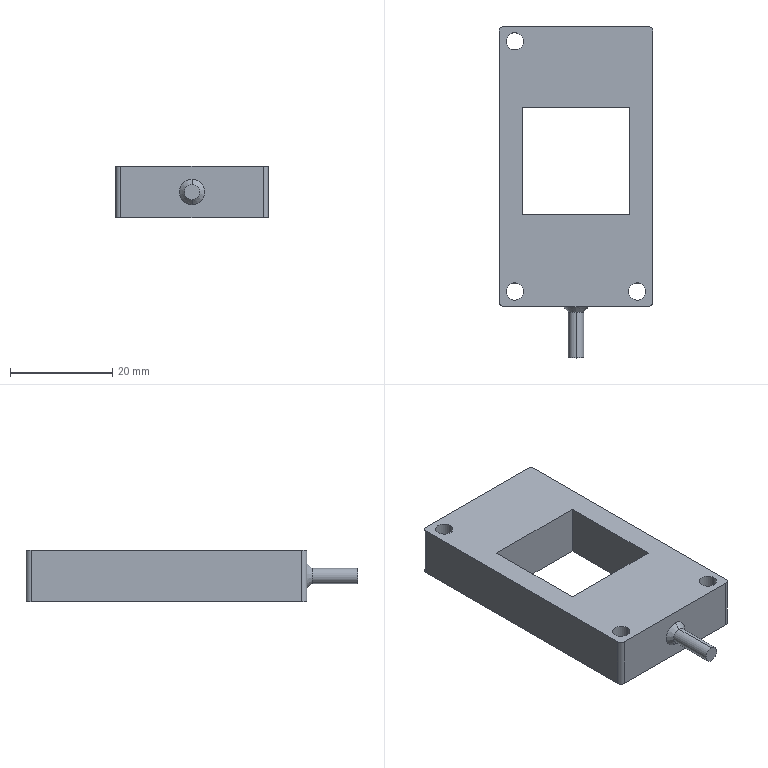Part | SolidWorks | features ICE 2, Chamfer 1, Extrusion 1, Fillet 1, HoleWzd 1 | 1 solid | 25 faces | box 30 x 65 x 10 mm | volume 11885 mm3 | cylinder 12 | plane 11 | cone 2 | commonest cylinder face diameters 3.4 x6 2 x4 3 x2
STEP:
#1=CARTESIAN_POINT('',(-13.7,24.5,-5.));
#2=VERTEX_POINT('',#1);
#3=CARTESIAN_POINT('',(-10.3,24.5,-5.));
#4=VERTEX_POINT('',#3);
#5=CARTESIAN_POINT('',(-12.,24.5,-5.));
#6=DIRECTION('',(0.,0.,1.));
#7=DIRECTION('',(1.,0.,0.));
#8=AXIS2_PLACEMENT_3D('',#5,#6,#7);
#9=CIRCLE('',#8,1.7);
#10=EDGE_CURVE('',#2,#4,#9,.T.);
#11=ORIENTED_EDGE('',*,*,#10,.F.);
#12=CARTESIAN_POINT('',(-13.7,24.5,5.));
#13=VERTEX_POINT('',#12);
#14=CARTESIAN_POINT('',(-13.7,24.5,5.));
#15=DIRECTION('',(0.,0.,1.));
#16=VECTOR('',#15,1000.);
#17=LINE('',#14,#16);
#18=EDGE_CURVE('',#2,#13,#17,.T.);
#19=ORIENTED_EDGE('',*,*,#18,.T.);
#20=CARTESIAN_POINT('',(-10.3,24.5,5.));
#21=VERTEX_POINT('',#20);
#22=CARTESIAN_POINT('',(-12.,24.5,5.));
#23=DIRECTION('',(0.,0.,1.));
#24=DIRECTION('',(1.,0.,0.));
#25=AXIS2_PLACEMENT_3D('',#22,#23,#24);
#26=CIRCLE('',#25,1.7);
#27=EDGE_CURVE('',#13,#21,#26,.T.);
#28=ORIENTED_EDGE('',*,*,#27,.T.);
#29=CARTESIAN_POINT('',(-10.3,24.5,5.));
#30=DIRECTION('',(0.,0.,1.));
#31=VECTOR('',#30,1000.);
#32=LINE('',#29,#31);
#33=EDGE_CURVE('',#4,#21,#32,.T.);
#34=ORIENTED_EDGE('',*,*,#33,.F.);
#35=EDGE_LOOP('',(#11,#19,#28,#34));
#36=FACE_OUTER_BOUND('',#35,.T.);
#37=CARTESIAN_POINT('',(-12.,24.5,5.));
#38=DIRECTION('',(0.,0.,1.));
#39=DIRECTION('',(1.,0.,0.));
#40=AXIS2_PLACEMENT_3D('',#37,#38,#39);
#41=CYLINDRICAL_SURFACE('',#40,1.7);
#42=ADVANCED_FACE('',(#36),#41,.F.);
#43=CARTESIAN_POINT('',(-13.7,-24.5,-5.));
#44=VERTEX_POINT('',#43);
#45=CARTESIAN_POINT('',(-10.3,-24.5,-5.));
#46=VERTEX_POINT('',#45);
#47=CARTESIAN_POINT('',(-12.,-24.5,-5.));
#48=DIRECTION('',(0.,0.,1.));
#49=DIRECTION('',(1.,0.,0.));
#50=AXIS2_PLACEMENT_3D('',#47,#48,#49);
#51=CIRCLE('',#50,1.7);
#52=EDGE_CURVE('',#44,#46,#51,.T.);
#53=ORIENTED_EDGE('',*,*,#52,.F.);
#54=CARTESIAN_POINT('',(-13.7,-24.5,5.));
#55=VERTEX_POINT('',#54);
#56=CARTESIAN_POINT('',(-13.7,-24.5,5.));
#57=DIRECTION('',(0.,0.,1.));
#58=VECTOR('',#57,1000.);
#59=LINE('',#56,#58);
#60=EDGE_CURVE('',#44,#55,#59,.T.);
#61=ORIENTED_EDGE('',*,*,#60,.T.);
#62=CARTESIAN_POINT('',(-10.3,-24.5,5.));
#63=VERTEX_POINT('',#62);
#64=CARTESIAN_POINT('',(-12.,-24.5,5.));
#65=DIRECTION('',(0.,0.,1.));
#66=DIRECTION('',(1.,0.,0.));
#67=AXIS2_PLACEMENT_3D('',#64,#65,#66);
#68=CIRCLE('',#67,1.7);
#69=EDGE_CURVE('',#55,#63,#68,.T.);
#70=ORIENTED_EDGE('',*,*,#69,.T.);
#71=CARTESIAN_POINT('',(-10.3,-24.5,5.));
#72=DIRECTION('',(0.,0.,1.));
#73=VECTOR('',#72,1000.);
#74=LINE('',#71,#73);
#75=EDGE_CURVE('',#46,#63,#74,.T.);
#76=ORIENTED_EDGE('',*,*,#75,.F.);
#77=EDGE_LOOP('',(#53,#61,#70,#76));
#78=FACE_OUTER_BOUND('',#77,.T.);
#79=CARTESIAN_POINT('',(-12.,-24.5,5.));
#80=DIRECTION('',(0.,0.,1.));
#81=DIRECTION('',(1.,0.,0.));
#82=AXIS2_PLACEMENT_3D('',#79,#80,#81);
#83=CYLINDRICAL_SURFACE('',#82,1.7);
#84=ADVANCED_FACE('',(#78),#83,.F.);
#85=CARTESIAN_POINT('',(10.3,-24.5,-5.));
#86=VERTEX_POINT('',#85);
#87=CARTESIAN_POINT('',(13.7,-24.5,-5.));
#88=VERTEX_POINT('',#87);
#89=CARTESIAN_POINT('',(12.,-24.5,-5.));
#90=DIRECTION('',(0.,0.,1.));
#91=DIRECTION('',(1.,0.,0.));
#92=AXIS2_PLACEMENT_3D('',#89,#90,#91);
#93=CIRCLE('',#92,1.7);
#94=EDGE_CURVE('',#86,#88,#93,.T.);
#95=ORIENTED_EDGE('',*,*,#94,.F.);
#96=CARTESIAN_POINT('',(10.3,-24.5,5.));
#97=VERTEX_POINT('',#96);
#98=CARTESIAN_POINT('',(10.3,-24.5,5.));
#99=DIRECTION('',(0.,0.,1.));
#100=VECTOR('',#99,1000.);
#101=LINE('',#98,#100);
#102=EDGE_CURVE('',#86,#97,#101,.T.);
#103=ORIENTED_EDGE('',*,*,#102,.T.);
#104=CARTESIAN_POINT('',(13.7,-24.5,5.));
#105=VERTEX_POINT('',#104);
#106=CARTESIAN_POINT('',(12.,-24.5,5.));
#107=DIRECTION('',(0.,0.,1.));
#108=DIRECTION('',(1.,0.,0.));
#109=AXIS2_PLACEMENT_3D('',#106,#107,#108);
#110=CIRCLE('',#109,1.7);
#111=EDGE_CURVE('',#97,#105,#110,.T.);
#112=ORIENTED_EDGE('',*,*,#111,.T.);
#113=CARTESIAN_POINT('',(13.7,-24.5,5.));
#114=DIRECTION('',(0.,0.,1.));
#115=VECTOR('',#114,1000.);
#116=LINE('',#113,#115);
#117=EDGE_CURVE('',#88,#105,#116,.T.);
#118=ORIENTED_EDGE('',*,*,#117,.F.);
#119=EDGE_LOOP('',(#95,#103,#112,#118));
#120=FACE_OUTER_BOUND('',#119,.T.);
#121=CARTESIAN_POINT('',(12.,-24.5,5.));
#122=DIRECTION('',(0.,0.,1.));
#123=DIRECTION('',(1.,0.,0.));
#124=AXIS2_PLACEMENT_3D('',#121,#122,#123);
#125=CYLINDRICAL_SURFACE('',#124,1.7);
#126=ADVANCED_FACE('',(#120),#125,.F.);
#127=CARTESIAN_POINT('',(0.,-28.5,-1.5));
#128=VERTEX_POINT('',#127);
#129=CARTESIAN_POINT('',(0.,-28.5,1.5));
#130=VERTEX_POINT('',#129);
#131=CARTESIAN_POINT('',(0.,-28.5,0.));
#132=DIRECTION('',(0.,-1.,0.));
#133=DIRECTION('',(0.,0.,1.));
#134=AXIS2_PLACEMENT_3D('',#131,#132,#133);
#135=CIRCLE('',#134,1.5);
#136=EDGE_CURVE('',#128,#130,#135,.T.);
#137=ORIENTED_EDGE('',*,*,#136,.F.);
#138=CARTESIAN_POINT('',(0.,-27.5,-2.5));
#139=VERTEX_POINT('',#138);
#140=CARTESIAN_POINT('',(0.,-28.5,-1.5));
#141=DIRECTION('',(0.,0.7071,-0.7071));
#142=VECTOR('',#141,1000.);
#143=LINE('',#140,#142);
#144=EDGE_CURVE('',#128,#139,#143,.T.);
#145=ORIENTED_EDGE('',*,*,#144,.T.);
#146=CARTESIAN_POINT('',(0.,-27.5,2.5));
#147=VERTEX_POINT('',#146);
#148=CARTESIAN_POINT('',(0.,-27.5,0.));
#149=DIRECTION('',(0.,1.,0.));
#150=DIRECTION('',(0.,0.,1.));
#151=AXIS2_PLACEMENT_3D('',#148,#149,#150);
#152=CIRCLE('',#151,2.5);
#153=EDGE_CURVE('',#147,#139,#152,.T.);
#154=ORIENTED_EDGE('',*,*,#153,.F.);
#155=CARTESIAN_POINT('',(0.,-28.5,1.5));
#156=DIRECTION('',(0.,0.7071,0.7071));
#157=VECTOR('',#156,1000.);
#158=LINE('',#155,#157);
#159=EDGE_CURVE('',#130,#147,#158,.T.);
#160=ORIENTED_EDGE('',*,*,#159,.F.);
#161=EDGE_LOOP('',(#137,#145,#154,#160));
#162=FACE_OUTER_BOUND('',#161,.T.);
#163=CARTESIAN_POINT('',(0.,-28.5,0.));
#164=DIRECTION('',(0.,1.,0.));
#165=DIRECTION('',(0.,0.,1.));
#166=AXIS2_PLACEMENT_3D('',#163,#164,#165);
#167=CONICAL_SURFACE('',#166,1.5,0.7854);
#168=ADVANCED_FACE('',(#162),#167,.T.);
#169=CARTESIAN_POINT('',(0.,-37.5,-1.5));
#170=VERTEX_POINT('',#169);
#171=CARTESIAN_POINT('',(0.,-37.5,1.5));
#172=VERTEX_POINT('',#171);
#173=CARTESIAN_POINT('',(0.,-37.5,0.));
#174=DIRECTION('',(0.,-1.,0.));
#175=DIRECTION('',(0.,0.,-1.));
#176=AXIS2_PLACEMENT_3D('',#173,#174,#175);
#177=CIRCLE('',#176,1.5);
#178=EDGE_CURVE('',#170,#172,#177,.T.);
#179=ORIENTED_EDGE('',*,*,#178,.F.);
#180=CARTESIAN_POINT('',(0.,-37.5,-1.5));
#181=DIRECTION('',(0.,1.,0.));
#182=VECTOR('',#181,1000.);
#183=LINE('',#180,#182);
#184=EDGE_CURVE('',#170,#128,#183,.T.);
#185=ORIENTED_EDGE('',*,*,#184,.T.);
#186=ORIENTED_EDGE('',*,*,#136,.T.);
#187=CARTESIAN_POINT('',(0.,-37.5,1.5));
#188=DIRECTION('',(0.,1.,0.));
#189=VECTOR('',#188,1000.);
#190=LINE('',#187,#189);
#191=EDGE_CURVE('',#172,#130,#190,.T.);
#192=ORIENTED_EDGE('',*,*,#191,.F.);
#193=EDGE_LOOP('',(#179,#185,#186,#192));
#194=FACE_OUTER_BOUND('',#193,.T.);
#195=CARTESIAN_POINT('',(0.,-37.5,0.));
#196=DIRECTION('',(0.,1.,0.));
#197=DIRECTION('',(0.,0.,1.));
#198=AXIS2_PLACEMENT_3D('',#195,#196,#197);
#199=CYLINDRICAL_SURFACE('',#198,1.5);
#200=ADVANCED_FACE('',(#194),#199,.T.);
#201=ORIENTED_EDGE('',*,*,#153,.T.);
#202=CARTESIAN_POINT('',(0.,-27.5,0.));
#203=DIRECTION('',(0.,1.,0.));
#204=DIRECTION('',(0.,0.,1.));
#205=AXIS2_PLACEMENT_3D('',#202,#203,#204);
#206=CIRCLE('',#205,2.5);
#207=EDGE_CURVE('',#139,#147,#206,.T.);
#208=ORIENTED_EDGE('',*,*,#207,.T.);
#209=EDGE_LOOP('',(#201,#208));
#210=FACE_BOUND('',#209,.T.);
#211=CARTESIAN_POINT('',(-14.,-27.5,5.));
#212=VERTEX_POINT('',#211);
#213=CARTESIAN_POINT('',(14.,-27.5,5.));
#214=VERTEX_POINT('',#213);
#215=CARTESIAN_POINT('',(-15.,-27.5,5.));
#216=DIRECTION('',(1.,0.,0.));
#217=VECTOR('',#216,1000.);
#218=LINE('',#215,#217);
#219=EDGE_CURVE('',#212,#214,#218,.T.);
#220=ORIENTED_EDGE('',*,*,#219,.F.);
#221=CARTESIAN_POINT('',(-14.,-27.5,-5.));
#222=VERTEX_POINT('',#221);
#223=CARTESIAN_POINT('',(-14.,-27.5,5.));
#224=DIRECTION('',(0.,0.,-1.));
#225=VECTOR('',#224,1000.);
#226=LINE('',#223,#225);
#227=EDGE_CURVE('',#212,#222,#226,.T.);
#228=ORIENTED_EDGE('',*,*,#227,.T.);
#229=CARTESIAN_POINT('',(14.,-27.5,-5.));
#230=VERTEX_POINT('',#229);
#231=CARTESIAN_POINT('',(-15.,-27.5,-5.));
#232=DIRECTION('',(1.,0.,0.));
#233=VECTOR('',#232,1000.);
#234=LINE('',#231,#233);
#235=EDGE_CURVE('',#222,#230,#234,.T.);
#236=ORIENTED_EDGE('',*,*,#235,.T.);
#237=CARTESIAN_POINT('',(14.,-27.5,5.));
#238=DIRECTION('',(0.,0.,1.));
#239=VECTOR('',#238,1000.);
#240=LINE('',#237,#239);
#241=EDGE_CURVE('',#230,#214,#240,.T.);
#242=ORIENTED_EDGE('',*,*,#241,.T.);
#243=EDGE_LOOP('',(#220,#228,#236,#242));
#244=FACE_OUTER_BOUND('',#243,.T.);
#245=CARTESIAN_POINT('',(-15.,-27.5,5.));
#246=DIRECTION('',(0.,1.,0.));
#247=DIRECTION('',(0.,0.,1.));
#248=AXIS2_PLACEMENT_3D('',#245,#246,#247);
#249=PLANE('',#248);
#250=ADVANCED_FACE('',(#210,#244),#249,.F.);
#251=CARTESIAN_POINT('',(15.,-26.5,5.));
#252=VERTEX_POINT('',#251);
#253=CARTESIAN_POINT('',(15.,26.5,5.));
#254=VERTEX_POINT('',#253);
#255=CARTESIAN_POINT('',(15.,27.5,5.));
#256=DIRECTION('',(0.,1.,0.));
#257=VECTOR('',#256,1000.);
#258=LINE('',#255,#257);
#259=EDGE_CURVE('',#252,#254,#258,.T.);
#260=ORIENTED_EDGE('',*,*,#259,.F.);
#261=CARTESIAN_POINT('',(15.,-26.5,-5.));
#262=VERTEX_POINT('',#261);
#263=CARTESIAN_POINT('',(15.,-26.5,5.));
#264=DIRECTION('',(0.,0.,-1.));
#265=VECTOR('',#264,1000.);
#266=LINE('',#263,#265);
#267=EDGE_CURVE('',#252,#262,#266,.T.);
#268=ORIENTED_EDGE('',*,*,#267,.T.);
#269=CARTESIAN_POINT('',(15.,26.5,-5.));
#270=VERTEX_POINT('',#269);
#271=CARTESIAN_POINT('',(15.,27.5,-5.));
#272=DIRECTION('',(0.,1.,0.));
#273=VECTOR('',#272,1000.);
#274=LINE('',#271,#273);
#275=EDGE_CURVE('',#262,#270,#274,.T.);
#276=ORIENTED_EDGE('',*,*,#275,.T.);
#277=CARTESIAN_POINT('',(15.,26.5,5.));
#278=DIRECTION('',(0.,0.,1.));
#279=VECTOR('',#278,1000.);
#280=LINE('',#277,#279);
#281=EDGE_CURVE('',#270,#254,#280,.T.);
#282=ORIENTED_EDGE('',*,*,#281,.T.);
#283=EDGE_LOOP('',(#260,#268,#276,#282));
#284=FACE_OUTER_BOUND('',#283,.T.);
#285=CARTESIAN_POINT('',(15.,27.5,5.));
#286=DIRECTION('',(-1.,0.,0.));
#287=DIRECTION('',(0.,-1.,0.));
#288=AXIS2_PLACEMENT_3D('',#285,#286,#287);
#289=PLANE('',#288);
#290=ADVANCED_FACE('',(#284),#289,.F.);
#291=CARTESIAN_POINT('',(14.,27.5,5.));
#292=VERTEX_POINT('',#291);
#293=CARTESIAN_POINT('',(-14.,27.5,5.));
#294=VERTEX_POINT('',#293);
#295=CARTESIAN_POINT('',(-15.,27.5,5.));
#296=DIRECTION('',(-1.,0.,0.));
#297=VECTOR('',#296,1000.);
#298=LINE('',#295,#297);
#299=EDGE_CURVE('',#292,#294,#298,.T.);
#300=ORIENTED_EDGE('',*,*,#299,.F.);
#301=CARTESIAN_POINT('',(14.,27.5,-5.));
#302=VERTEX_POINT('',#301);
#303=CARTESIAN_POINT('',(14.,27.5,5.));
#304=DIRECTION('',(0.,0.,-1.));
#305=VECTOR('',#304,1000.);
#306=LINE('',#303,#305);
#307=EDGE_CURVE('',#292,#302,#306,.T.);
#308=ORIENTED_EDGE('',*,*,#307,.T.);
#309=CARTESIAN_POINT('',(-14.,27.5,-5.));
#310=VERTEX_POINT('',#309);
#311=CARTESIAN_POINT('',(-15.,27.5,-5.));
#312=DIRECTION('',(-1.,0.,0.));
#313=VECTOR('',#312,1000.);
#314=LINE('',#311,#313);
#315=EDGE_CURVE('',#302,#310,#314,.T.);
#316=ORIENTED_EDGE('',*,*,#315,.T.);
#317=CARTESIAN_POINT('',(-14.,27.5,5.));
#318=DIRECTION('',(0.,0.,1.));
#319=VECTOR('',#318,1000.);
#320=LINE('',#317,#319);
#321=EDGE_CURVE('',#310,#294,#320,.T.);
#322=ORIENTED_EDGE('',*,*,#321,.T.);
#323=EDGE_LOOP('',(#300,#308,#316,#322));
#324=FACE_OUTER_BOUND('',#323,.T.);
#325=CARTESIAN_POINT('',(-15.,27.5,5.));
#326=DIRECTION('',(0.,-1.,0.));
#327=DIRECTION('',(0.,0.,-1.));
#328=AXIS2_PLACEMENT_3D('',#325,#326,#327);
#329=PLANE('',#328);
#330=ADVANCED_FACE('',(#324),#329,.F.);
#331=CARTESIAN_POINT('',(-15.,26.5,-5.));
#332=VERTEX_POINT('',#331);
#333=CARTESIAN_POINT('',(-15.,-26.5,-5.));
#334=VERTEX_POINT('',#333);
#335=CARTESIAN_POINT('',(-15.,27.5,-5.));
#336=DIRECTION('',(0.,-1.,0.));
#337=VECTOR('',#336,1000.);
#338=LINE('',#335,#337);
#339=EDGE_CURVE('',#332,#334,#338,.T.);
#340=ORIENTED_EDGE('',*,*,#339,.T.);
#341=CARTESIAN_POINT('',(-15.,-26.5,5.));
#342=VERTEX_POINT('',#341);
#343=CARTESIAN_POINT('',(-15.,-26.5,5.));
#344=DIRECTION('',(0.,0.,1.));
#345=VECTOR('',#344,1000.);
#346=LINE('',#343,#345);
#347=EDGE_CURVE('',#334,#342,#346,.T.);
#348=ORIENTED_EDGE('',*,*,#347,.T.);
#349=CARTESIAN_POINT('',(-15.,26.5,5.));
#350=VERTEX_POINT('',#349);
#351=CARTESIAN_POINT('',(-15.,27.5,5.));
#352=DIRECTION('',(0.,-1.,0.));
#353=VECTOR('',#352,1000.);
#354=LINE('',#351,#353);
#355=EDGE_CURVE('',#350,#342,#354,.T.);
#356=ORIENTED_EDGE('',*,*,#355,.F.);
#357=CARTESIAN_POINT('',(-15.,26.5,5.));
#358=DIRECTION('',(0.,0.,-1.));
#359=VECTOR('',#358,1000.);
#360=LINE('',#357,#359);
#361=EDGE_CURVE('',#350,#332,#360,.T.);
#362=ORIENTED_EDGE('',*,*,#361,.T.);
#363=EDGE_LOOP('',(#340,#348,#356,#362));
#364=FACE_OUTER_BOUND('',#363,.T.);
#365=CARTESIAN_POINT('',(-15.,27.5,5.));
#366=DIRECTION('',(1.,0.,0.));
#367=DIRECTION('',(0.,1.,0.));
#368=AXIS2_PLACEMENT_3D('',#365,#366,#367);
#369=PLANE('',#368);
#370=ADVANCED_FACE('',(#364),#369,.F.);
#371=CARTESIAN_POINT('',(-12.,24.5,5.));
#372=DIRECTION('',(0.,0.,1.));
#373=DIRECTION('',(1.,0.,0.));
#374=AXIS2_PLACEMENT_3D('',#371,#372,#373);
#375=CIRCLE('',#374,1.7);
#376=EDGE_CURVE('',#21,#13,#375,.T.);
#377=ORIENTED_EDGE('',*,*,#376,.F.);
#378=ORIENTED_EDGE('',*,*,#27,.F.);
#379=EDGE_LOOP('',(#377,#378));
#380=FACE_BOUND('',#379,.T.);
#381=CARTESIAN_POINT('',(-12.,-24.5,5.));
#382=DIRECTION('',(0.,0.,1.));
#383=DIRECTION('',(1.,0.,0.));
#384=AXIS2_PLACEMENT_3D('',#381,#382,#383);
#385=CIRCLE('',#384,1.7);
#386=EDGE_CURVE('',#63,#55,#385,.T.);
#387=ORIENTED_EDGE('',*,*,#386,.F.);
#388=ORIENTED_EDGE('',*,*,#69,.F.);
#389=EDGE_LOOP('',(#387,#388));
#390=FACE_BOUND('',#389,.T.);
#391=CARTESIAN_POINT('',(12.,-24.5,5.));
#392=DIRECTION('',(0.,0.,1.));
#393=DIRECTION('',(1.,0.,0.));
#394=AXIS2_PLACEMENT_3D('',#391,#392,#393);
#395=CIRCLE('',#394,1.7);
#396=EDGE_CURVE('',#105,#97,#395,.T.);
#397=ORIENTED_EDGE('',*,*,#396,.F.);
#398=ORIENTED_EDGE('',*,*,#111,.F.);
#399=EDGE_LOOP('',(#397,#398));
#400=FACE_BOUND('',#399,.T.);
#401=CARTESIAN_POINT('',(10.5,-9.5,5.));
#402=VERTEX_POINT('',#401);
#403=CARTESIAN_POINT('',(10.5,11.5,5.));
#404=VERTEX_POINT('',#403);
#405=CARTESIAN_POINT('',(10.5,11.5,5.));
#406=DIRECTION('',(0.,1.,0.));
#407=VECTOR('',#406,1000.);
#408=LINE('',#405,#407);
#409=EDGE_CURVE('',#402,#404,#408,.T.);
#410=ORIENTED_EDGE('',*,*,#409,.F.);
#411=CARTESIAN_POINT('',(-10.5,-9.5,5.));
#412=VERTEX_POINT('',#411);
#413=CARTESIAN_POINT('',(-10.5,-9.5,5.));
#414=DIRECTION('',(1.,0.,0.));
#415=VECTOR('',#414,1000.);
#416=LINE('',#413,#415);
#417=EDGE_CURVE('',#412,#402,#416,.T.);
#418=ORIENTED_EDGE('',*,*,#417,.F.);
#419=CARTESIAN_POINT('',(-10.5,11.5,5.));
#420=VERTEX_POINT('',#419);
#421=CARTESIAN_POINT('',(-10.5,11.5,5.));
#422=DIRECTION('',(0.,-1.,0.));
#423=VECTOR('',#422,1000.);
#424=LINE('',#421,#423);
#425=EDGE_CURVE('',#420,#412,#424,.T.);
#426=ORIENTED_EDGE('',*,*,#425,.F.);
#427=CARTESIAN_POINT('',(-10.5,11.5,5.));
#428=DIRECTION('',(-1.,0.,0.));
#429=VECTOR('',#428,1000.);
#430=LINE('',#427,#429);
#431=EDGE_CURVE('',#404,#420,#430,.T.);
#432=ORIENTED_EDGE('',*,*,#431,.F.);
#433=EDGE_LOOP('',(#410,#418,#426,#432));
#434=FACE_BOUND('',#433,.T.);
#435=ORIENTED_EDGE('',*,*,#355,.T.);
#436=CARTESIAN_POINT('',(-14.,-26.5,5.));
#437=DIRECTION('',(0.,0.,1.));
#438=DIRECTION('',(1.,0.,0.));
#439=AXIS2_PLACEMENT_3D('',#436,#437,#438);
#440=CIRCLE('',#439,1.);
#441=EDGE_CURVE('',#342,#212,#440,.T.);
#442=ORIENTED_EDGE('',*,*,#441,.T.);
#443=ORIENTED_EDGE('',*,*,#219,.T.);
#444=CARTESIAN_POINT('',(14.,-26.5,5.));
#445=DIRECTION('',(0.,0.,1.));
#446=DIRECTION('',(1.,0.,0.));
#447=AXIS2_PLACEMENT_3D('',#444,#445,#446);
#448=CIRCLE('',#447,1.);
#449=EDGE_CURVE('',#214,#252,#448,.T.);
#450=ORIENTED_EDGE('',*,*,#449,.T.);
#451=ORIENTED_EDGE('',*,*,#259,.T.);
#452=CARTESIAN_POINT('',(14.,26.5,5.));
#453=DIRECTION('',(0.,0.,1.));
#454=DIRECTION('',(1.,0.,0.));
#455=AXIS2_PLACEMENT_3D('',#452,#453,#454);
#456=CIRCLE('',#455,1.);
#457=EDGE_CURVE('',#254,#292,#456,.T.);
#458=ORIENTED_EDGE('',*,*,#457,.T.);
#459=ORIENTED_EDGE('',*,*,#299,.T.);
#460=CARTESIAN_POINT('',(-14.,26.5,5.));
#461=DIRECTION('',(0.,0.,1.));
#462=DIRECTION('',(1.,0.,0.));
#463=AXIS2_PLACEMENT_3D('',#460,#461,#462);
#464=CIRCLE('',#463,1.);
#465=EDGE_CURVE('',#294,#350,#464,.T.);
#466=ORIENTED_EDGE('',*,*,#465,.T.);
#467=EDGE_LOOP('',(#435,#442,#443,#450,#451,#458,#459,#466));
#468=FACE_OUTER_BOUND('',#467,.T.);
#469=CARTESIAN_POINT('',(0.,0.,5.));
#470=DIRECTION('',(0.,0.,1.));
#471=DIRECTION('',(1.,0.,0.));
#472=AXIS2_PLACEMENT_3D('',#469,#470,#471);
#473=PLANE('',#472);
#474=ADVANCED_FACE('',(#380,#390,#400,#434,#468),#473,.T.);
#475=CARTESIAN_POINT('',(-12.,24.5,-5.));
#476=DIRECTION('',(0.,0.,1.));
#477=DIRECTION('',(1.,0.,0.));
#478=AXIS2_PLACEMENT_3D('',#475,#476,#477);
#479=CIRCLE('',#478,1.7);
#480=EDGE_CURVE('',#4,#2,#479,.T.);
#481=ORIENTED_EDGE('',*,*,#480,.T.);
#482=ORIENTED_EDGE('',*,*,#10,.T.);
#483=EDGE_LOOP('',(#481,#482));
#484=FACE_BOUND('',#483,.T.);
#485=CARTESIAN_POINT('',(-12.,-24.5,-5.));
#486=DIRECTION('',(0.,0.,1.));
#487=DIRECTION('',(1.,0.,0.));
#488=AXIS2_PLACEMENT_3D('',#485,#486,#487);
#489=CIRCLE('',#488,1.7);
#490=EDGE_CURVE('',#46,#44,#489,.T.);
#491=ORIENTED_EDGE('',*,*,#490,.T.);
#492=ORIENTED_EDGE('',*,*,#52,.T.);
#493=EDGE_LOOP('',(#491,#492));
#494=FACE_BOUND('',#493,.T.);
#495=CARTESIAN_POINT('',(12.,-24.5,-5.));
#496=DIRECTION('',(0.,0.,1.));
#497=DIRECTION('',(1.,0.,0.));
#498=AXIS2_PLACEMENT_3D('',#495,#496,#497);
#499=CIRCLE('',#498,1.7);
#500=EDGE_CURVE('',#88,#86,#499,.T.);
#501=ORIENTED_EDGE('',*,*,#500,.T.);
#502=ORIENTED_EDGE('',*,*,#94,.T.);
#503=EDGE_LOOP('',(#501,#502));
#504=FACE_BOUND('',#503,.T.);
#505=CARTESIAN_POINT('',(-10.5,-9.5,-5.));
#506=VERTEX_POINT('',#505);
#507=CARTESIAN_POINT('',(10.5,-9.5,-5.));
#508=VERTEX_POINT('',#507);
#509=CARTESIAN_POINT('',(-10.5,-9.5,-5.));
#510=DIRECTION('',(1.,0.,0.));
#511=VECTOR('',#510,1000.);
#512=LINE('',#509,#511);
#513=EDGE_CURVE('',#506,#508,#512,.T.);
#514=ORIENTED_EDGE('',*,*,#513,.T.);
#515=CARTESIAN_POINT('',(10.5,11.5,-5.));
#516=VERTEX_POINT('',#515);
#517=CARTESIAN_POINT('',(10.5,11.5,-5.));
#518=DIRECTION('',(0.,1.,0.));
#519=VECTOR('',#518,1000.);
#520=LINE('',#517,#519);
#521=EDGE_CURVE('',#508,#516,#520,.T.);
#522=ORIENTED_EDGE('',*,*,#521,.T.);
#523=CARTESIAN_POINT('',(-10.5,11.5,-5.));
#524=VERTEX_POINT('',#523);
#525=CARTESIAN_POINT('',(-10.5,11.5,-5.));
#526=DIRECTION('',(-1.,0.,0.));
#527=VECTOR('',#526,1000.);
#528=LINE('',#525,#527);
#529=EDGE_CURVE('',#516,#524,#528,.T.);
#530=ORIENTED_EDGE('',*,*,#529,.T.);
#531=CARTESIAN_POINT('',(-10.5,11.5,-5.));
#532=DIRECTION('',(0.,-1.,0.));
#533=VECTOR('',#532,1000.);
#534=LINE('',#531,#533);
#535=EDGE_CURVE('',#524,#506,#534,.T.);
#536=ORIENTED_EDGE('',*,*,#535,.T.);
#537=EDGE_LOOP('',(#514,#522,#530,#536));
#538=FACE_BOUND('',#537,.T.);
#539=ORIENTED_EDGE('',*,*,#235,.F.);
#540=CARTESIAN_POINT('',(-14.,-26.5,-5.));
#541=DIRECTION('',(0.,0.,-1.));
#542=DIRECTION('',(1.,0.,0.));
#543=AXIS2_PLACEMENT_3D('',#540,#541,#542);
#544=CIRCLE('',#543,1.);
#545=EDGE_CURVE('',#222,#334,#544,.T.);
#546=ORIENTED_EDGE('',*,*,#545,.T.);
#547=ORIENTED_EDGE('',*,*,#339,.F.);
#548=CARTESIAN_POINT('',(-14.,26.5,-5.));
#549=DIRECTION('',(0.,0.,-1.));
#550=DIRECTION('',(1.,0.,0.));
#551=AXIS2_PLACEMENT_3D('',#548,#549,#550);
#552=CIRCLE('',#551,1.);
#553=EDGE_CURVE('',#332,#310,#552,.T.);
#554=ORIENTED_EDGE('',*,*,#553,.T.);
#555=ORIENTED_EDGE('',*,*,#315,.F.);
#556=CARTESIAN_POINT('',(14.,26.5,-5.));
#557=DIRECTION('',(0.,0.,-1.));
#558=DIRECTION('',(1.,0.,0.));
#559=AXIS2_PLACEMENT_3D('',#556,#557,#558);
#560=CIRCLE('',#559,1.);
#561=EDGE_CURVE('',#302,#270,#560,.T.);
#562=ORIENTED_EDGE('',*,*,#561,.T.);
#563=ORIENTED_EDGE('',*,*,#275,.F.);
#564=CARTESIAN_POINT('',(14.,-26.5,-5.));
#565=DIRECTION('',(0.,0.,-1.));
#566=DIRECTION('',(1.,0.,0.));
#567=AXIS2_PLACEMENT_3D('',#564,#565,#566);
#568=CIRCLE('',#567,1.);
#569=EDGE_CURVE('',#262,#230,#568,.T.);
#570=ORIENTED_EDGE('',*,*,#569,.T.);
#571=EDGE_LOOP('',(#539,#546,#547,#554,#555,#562,#563,#570));
#572=FACE_OUTER_BOUND('',#571,.T.);
#573=CARTESIAN_POINT('',(0.,0.,-5.));
#574=DIRECTION('',(0.,0.,1.));
#575=DIRECTION('',(1.,0.,0.));
#576=AXIS2_PLACEMENT_3D('',#573,#574,#575);
#577=PLANE('',#576);
#578=ADVANCED_FACE('',(#484,#494,#504,#538,#572),#577,.F.);
#579=ORIENTED_EDGE('',*,*,#409,.T.);
#580=CARTESIAN_POINT('',(10.5,11.5,-5.));
#581=DIRECTION('',(0.,0.,1.));
#582=VECTOR('',#581,1000.);
#583=LINE('',#580,#582);
#584=EDGE_CURVE('',#516,#404,#583,.T.);
#585=ORIENTED_EDGE('',*,*,#584,.F.);
#586=ORIENTED_EDGE('',*,*,#521,.F.);
#587=CARTESIAN_POINT('',(10.5,-9.5,-5.));
#588=DIRECTION('',(0.,0.,1.));
#589=VECTOR('',#588,1000.);
#590=LINE('',#587,#589);
#591=EDGE_CURVE('',#508,#402,#590,.T.);
#592=ORIENTED_EDGE('',*,*,#591,.T.);
#593=EDGE_LOOP('',(#579,#585,#586,#592));
#594=FACE_OUTER_BOUND('',#593,.T.);
#595=CARTESIAN_POINT('',(10.5,11.5,-5.));
#596=DIRECTION('',(1.,0.,0.));
#597=DIRECTION('',(0.,1.,0.));
#598=AXIS2_PLACEMENT_3D('',#595,#596,#597);
#599=PLANE('',#598);
#600=ADVANCED_FACE('',(#594),#599,.F.);
#601=ORIENTED_EDGE('',*,*,#417,.T.);
#602=ORIENTED_EDGE('',*,*,#591,.F.);
#603=ORIENTED_EDGE('',*,*,#513,.F.);
#604=CARTESIAN_POINT('',(-10.5,-9.5,-5.));
#605=DIRECTION('',(0.,0.,1.));
#606=VECTOR('',#605,1000.);
#607=LINE('',#604,#606);
#608=EDGE_CURVE('',#506,#412,#607,.T.);
#609=ORIENTED_EDGE('',*,*,#608,.T.);
#610=EDGE_LOOP('',(#601,#602,#603,#609));
#611=FACE_OUTER_BOUND('',#610,.T.);
#612=CARTESIAN_POINT('',(-10.5,-9.5,-5.));
#613=DIRECTION('',(0.,-1.,0.));
#614=DIRECTION('',(0.,0.,-1.));
#615=AXIS2_PLACEMENT_3D('',#612,#613,#614);
#616=PLANE('',#615);
#617=ADVANCED_FACE('',(#611),#616,.F.);
#618=ORIENTED_EDGE('',*,*,#425,.T.);
#619=ORIENTED_EDGE('',*,*,#608,.F.);
#620=ORIENTED_EDGE('',*,*,#535,.F.);
#621=CARTESIAN_POINT('',(-10.5,11.5,-5.));
#622=DIRECTION('',(0.,0.,1.));
#623=VECTOR('',#622,1000.);
#624=LINE('',#621,#623);
#625=EDGE_CURVE('',#524,#420,#624,.T.);
#626=ORIENTED_EDGE('',*,*,#625,.T.);
#627=EDGE_LOOP('',(#618,#619,#620,#626));
#628=FACE_OUTER_BOUND('',#627,.T.);
#629=CARTESIAN_POINT('',(-10.5,11.5,-5.));
#630=DIRECTION('',(-1.,0.,0.));
#631=DIRECTION('',(0.,-1.,0.));
#632=AXIS2_PLACEMENT_3D('',#629,#630,#631);
#633=PLANE('',#632);
#634=ADVANCED_FACE('',(#628),#633,.F.);
#635=ORIENTED_EDGE('',*,*,#431,.T.);
#636=ORIENTED_EDGE('',*,*,#625,.F.);
#637=ORIENTED_EDGE('',*,*,#529,.F.);
#638=ORIENTED_EDGE('',*,*,#584,.T.);
#639=EDGE_LOOP('',(#635,#636,#637,#638));
#640=FACE_OUTER_BOUND('',#639,.T.);
#641=CARTESIAN_POINT('',(-10.5,11.5,-5.));
#642=DIRECTION('',(0.,1.,0.));
#643=DIRECTION('',(0.,0.,1.));
#644=AXIS2_PLACEMENT_3D('',#641,#642,#643);
#645=PLANE('',#644);
#646=ADVANCED_FACE('',(#640),#645,.F.);
#647=ORIENTED_EDGE('',*,*,#184,.F.);
#648=CARTESIAN_POINT('',(0.,-37.5,0.));
#649=DIRECTION('',(0.,-1.,0.));
#650=DIRECTION('',(0.,0.,-1.));
#651=AXIS2_PLACEMENT_3D('',#648,#649,#650);
#652=CIRCLE('',#651,1.5);
#653=EDGE_CURVE('',#172,#170,#652,.T.);
#654=ORIENTED_EDGE('',*,*,#653,.F.);
#655=ORIENTED_EDGE('',*,*,#191,.T.);
#656=CARTESIAN_POINT('',(0.,-28.5,0.));
#657=DIRECTION('',(0.,-1.,0.));
#658=DIRECTION('',(0.,0.,1.));
#659=AXIS2_PLACEMENT_3D('',#656,#657,#658);
#660=CIRCLE('',#659,1.5);
#661=EDGE_CURVE('',#130,#128,#660,.T.);
#662=ORIENTED_EDGE('',*,*,#661,.T.);
#663=EDGE_LOOP('',(#647,#654,#655,#662));
#664=FACE_OUTER_BOUND('',#663,.T.);
#665=CARTESIAN_POINT('',(0.,-37.5,0.));
#666=DIRECTION('',(0.,1.,0.));
#667=DIRECTION('',(0.,0.,1.));
#668=AXIS2_PLACEMENT_3D('',#665,#666,#667);
#669=CYLINDRICAL_SURFACE('',#668,1.5);
#670=ADVANCED_FACE('',(#664),#669,.T.);
#671=ORIENTED_EDGE('',*,*,#653,.T.);
#672=ORIENTED_EDGE('',*,*,#178,.T.);
#673=EDGE_LOOP('',(#671,#672));
#674=FACE_OUTER_BOUND('',#673,.T.);
#675=CARTESIAN_POINT('',(0.,-37.5,0.));
#676=DIRECTION('',(0.,-1.,0.));
#677=DIRECTION('',(0.,0.,-1.));
#678=AXIS2_PLACEMENT_3D('',#675,#676,#677);
#679=PLANE('',#678);
#680=ADVANCED_FACE('',(#674),#679,.T.);
#681=ORIENTED_EDGE('',*,*,#144,.F.);
#682=ORIENTED_EDGE('',*,*,#661,.F.);
#683=ORIENTED_EDGE('',*,*,#159,.T.);
#684=ORIENTED_EDGE('',*,*,#207,.F.);
#685=EDGE_LOOP('',(#681,#682,#683,#684));
#686=FACE_OUTER_BOUND('',#685,.T.);
#687=CARTESIAN_POINT('',(0.,-28.5,0.));
#688=DIRECTION('',(0.,1.,0.));
#689=DIRECTION('',(0.,0.,1.));
#690=AXIS2_PLACEMENT_3D('',#687,#688,#689);
#691=CONICAL_SURFACE('',#690,1.5,0.7854);
#692=ADVANCED_FACE('',(#686),#691,.T.);
#693=ORIENTED_EDGE('',*,*,#441,.F.);
#694=ORIENTED_EDGE('',*,*,#347,.F.);
#695=ORIENTED_EDGE('',*,*,#545,.F.);
#696=ORIENTED_EDGE('',*,*,#227,.F.);
#697=EDGE_LOOP('',(#693,#694,#695,#696));
#698=FACE_OUTER_BOUND('',#697,.T.);
#699=CARTESIAN_POINT('',(-14.,-26.5,5.));
#700=DIRECTION('',(0.,0.,-1.));
#701=DIRECTION('',(-1.,0.,0.));
#702=AXIS2_PLACEMENT_3D('',#699,#700,#701);
#703=CYLINDRICAL_SURFACE('',#702,1.);
#704=ADVANCED_FACE('',(#698),#703,.T.);
#705=ORIENTED_EDGE('',*,*,#449,.F.);
#706=ORIENTED_EDGE('',*,*,#241,.F.);
#707=ORIENTED_EDGE('',*,*,#569,.F.);
#708=ORIENTED_EDGE('',*,*,#267,.F.);
#709=EDGE_LOOP('',(#705,#706,#707,#708));
#710=FACE_OUTER_BOUND('',#709,.T.);
#711=CARTESIAN_POINT('',(14.,-26.5,5.));
#712=DIRECTION('',(0.,0.,-1.));
#713=DIRECTION('',(-1.,0.,0.));
#714=AXIS2_PLACEMENT_3D('',#711,#712,#713);
#715=CYLINDRICAL_SURFACE('',#714,1.);
#716=ADVANCED_FACE('',(#710),#715,.T.);
#717=ORIENTED_EDGE('',*,*,#457,.F.);
#718=ORIENTED_EDGE('',*,*,#281,.F.);
#719=ORIENTED_EDGE('',*,*,#561,.F.);
#720=ORIENTED_EDGE('',*,*,#307,.F.);
#721=EDGE_LOOP('',(#717,#718,#719,#720));
#722=FACE_OUTER_BOUND('',#721,.T.);
#723=CARTESIAN_POINT('',(14.,26.5,5.));
#724=DIRECTION('',(0.,0.,-1.));
#725=DIRECTION('',(-1.,0.,0.));
#726=AXIS2_PLACEMENT_3D('',#723,#724,#725);
#727=CYLINDRICAL_SURFACE('',#726,1.);
#728=ADVANCED_FACE('',(#722),#727,.T.);
#729=ORIENTED_EDGE('',*,*,#465,.F.);
#730=ORIENTED_EDGE('',*,*,#321,.F.);
#731=ORIENTED_EDGE('',*,*,#553,.F.);
#732=ORIENTED_EDGE('',*,*,#361,.F.);
#733=EDGE_LOOP('',(#729,#730,#731,#732));
#734=FACE_OUTER_BOUND('',#733,.T.);
#735=CARTESIAN_POINT('',(-14.,26.5,5.));
#736=DIRECTION('',(0.,0.,-1.));
#737=DIRECTION('',(-1.,0.,0.));
#738=AXIS2_PLACEMENT_3D('',#735,#736,#737);
#739=CYLINDRICAL_SURFACE('',#738,1.);
#740=ADVANCED_FACE('',(#734),#739,.T.);
#741=ORIENTED_EDGE('',*,*,#102,.F.);
#742=ORIENTED_EDGE('',*,*,#500,.F.);
#743=ORIENTED_EDGE('',*,*,#117,.T.);
#744=ORIENTED_EDGE('',*,*,#396,.T.);
#745=EDGE_LOOP('',(#741,#742,#743,#744));
#746=FACE_OUTER_BOUND('',#745,.T.);
#747=CARTESIAN_POINT('',(12.,-24.5,5.));
#748=DIRECTION('',(0.,0.,1.));
#749=DIRECTION('',(1.,0.,0.));
#750=AXIS2_PLACEMENT_3D('',#747,#748,#749);
#751=CYLINDRICAL_SURFACE('',#750,1.7);
#752=ADVANCED_FACE('',(#746),#751,.F.);
#753=ORIENTED_EDGE('',*,*,#60,.F.);
#754=ORIENTED_EDGE('',*,*,#490,.F.);
#755=ORIENTED_EDGE('',*,*,#75,.T.);
#756=ORIENTED_EDGE('',*,*,#386,.T.);
#757=EDGE_LOOP('',(#753,#754,#755,#756));
#758=FACE_OUTER_BOUND('',#757,.T.);
#759=CARTESIAN_POINT('',(-12.,-24.5,5.));
#760=DIRECTION('',(0.,0.,1.));
#761=DIRECTION('',(1.,0.,0.));
#762=AXIS2_PLACEMENT_3D('',#759,#760,#761);
#763=CYLINDRICAL_SURFACE('',#762,1.7);
#764=ADVANCED_FACE('',(#758),#763,.F.);
#765=ORIENTED_EDGE('',*,*,#18,.F.);
#766=ORIENTED_EDGE('',*,*,#480,.F.);
#767=ORIENTED_EDGE('',*,*,#33,.T.);
#768=ORIENTED_EDGE('',*,*,#376,.T.);
#769=EDGE_LOOP('',(#765,#766,#767,#768));
#770=FACE_OUTER_BOUND('',#769,.T.);
#771=CARTESIAN_POINT('',(-12.,24.5,5.));
#772=DIRECTION('',(0.,0.,1.));
#773=DIRECTION('',(1.,0.,0.));
#774=AXIS2_PLACEMENT_3D('',#771,#772,#773);
#775=CYLINDRICAL_SURFACE('',#774,1.7);
#776=ADVANCED_FACE('',(#770),#775,.F.);
#777=CLOSED_SHELL('',(#42,#84,#126,#168,#200,#250,#290,#330,#370,#474,#578,#600,#617,#634,#646,#670,#680,#692,#704,#716,#728,#740,#752,#764,#776));
#778=MANIFOLD_SOLID_BREP('',#777);
#779=CARTESIAN_POINT('',(0.,0.,0.));
#780=DIRECTION('',(0.,0.,1.));
#781=DIRECTION('',(1.,0.,0.));
#782=AXIS2_PLACEMENT_3D('',#779,#780,#781);
#783=(LENGTH_UNIT()NAMED_UNIT(*)SI_UNIT(.MILLI.,.METRE.));
#784=UNCERTAINTY_MEASURE_WITH_UNIT(LENGTH_MEASURE(0.00001),#783,'','');
#785=(NAMED_UNIT(*)PLANE_ANGLE_UNIT()SI_UNIT($,.RADIAN.));
#786=(NAMED_UNIT(*)SI_UNIT($,.STERADIAN.)SOLID_ANGLE_UNIT());
#787=(GEOMETRIC_REPRESENTATION_CONTEXT(3)GLOBAL_UNCERTAINTY_ASSIGNED_CONTEXT((#784))GLOBAL_UNIT_ASSIGNED_CONTEXT((#783,#785,#786))REPRESENTATION_CONTEXT('',''));
#788=ADVANCED_BREP_SHAPE_REPRESENTATION('',(#778,#782),#787);